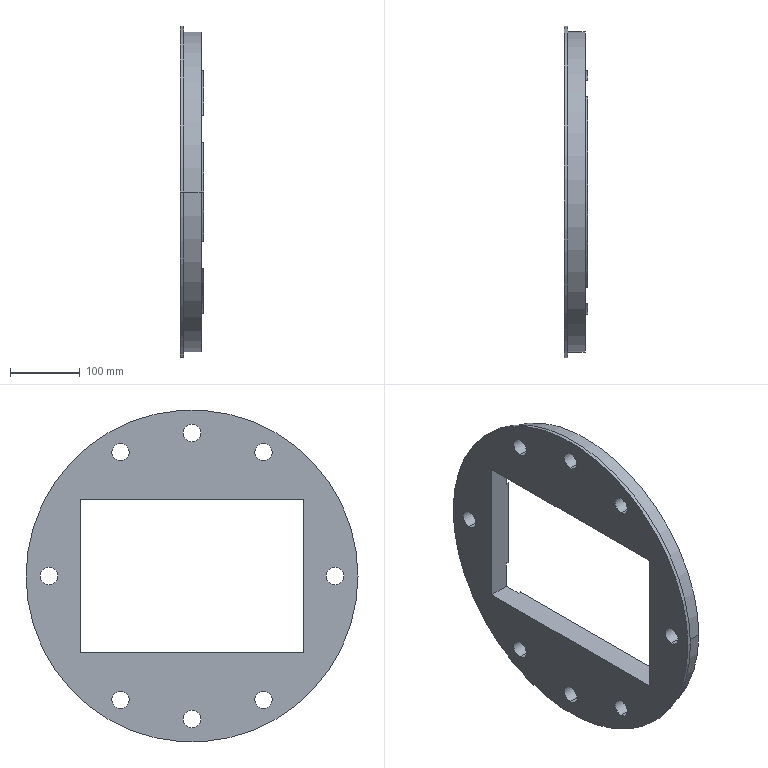Part | STEP file | Flange | 1 solid | 36 faces | box 34 x 476 x 476 mm | volume 2924692 mm3 | cylinder 25 | plane 11 | commonest cylinder face diameters 25 x16 350 x5 460 x2 476 x2